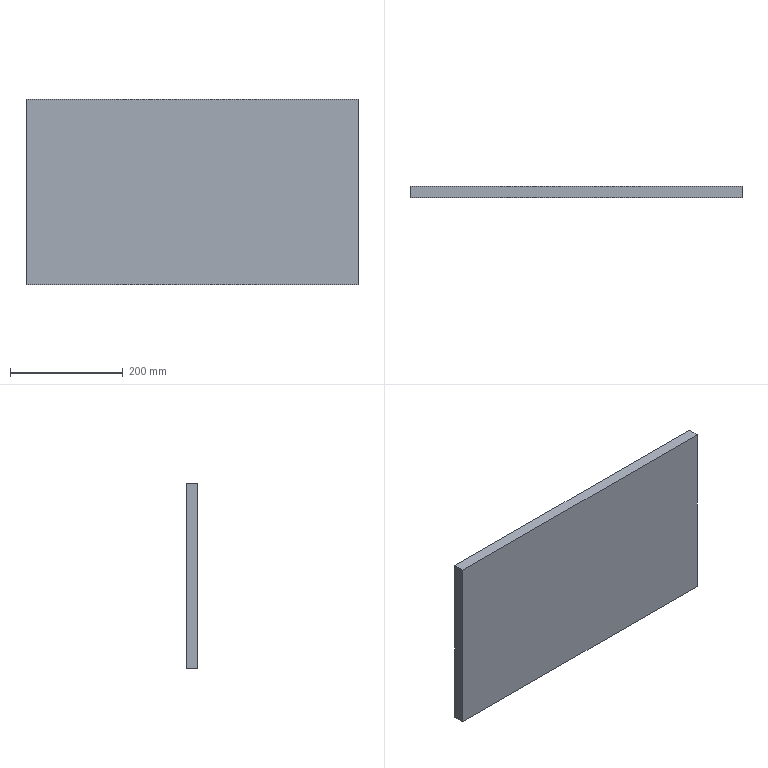Part | STEP file | Light guide plate 001 | 1 solid | 6 faces | box 590 x 20 x 330 mm | volume 3894000 mm3 | plane 6
STEP:
#1=CARTESIAN_POINT('',(0.,0.,0.));
#2=DIRECTION('',(0.,0.,1.));
#3=DIRECTION('',(1.,0.,0.));
#4=AXIS2_PLACEMENT_3D('',#1,#2,#3);
#5=CARTESIAN_POINT('',(295.,0.,165.));
#6=VERTEX_POINT('',#5);
#7=CARTESIAN_POINT('',(295.,0.,-165.));
#8=VERTEX_POINT('',#7);
#9=CARTESIAN_POINT('',(295.,0.,165.));
#10=DIRECTION('',(0.,0.,-1.));
#11=VECTOR('',#10,1.);
#12=LINE('',#9,#11);
#13=CARTESIAN_POINT('',(295.,20.,165.));
#14=DIRECTION('',(-1.,0.,0.));
#15=DIRECTION('',(0.,0.,1.));
#16=AXIS2_PLACEMENT_3D('',#13,#14,#15);
#17=PLANE('',#16);
#18=CARTESIAN_POINT('',(0.,-20.));
#19=DIRECTION('',(-1.,0.));
#20=VECTOR('',#19,1.);
#21=LINE('',#18,#20);
#22=(GEOMETRIC_REPRESENTATION_CONTEXT(2)PARAMETRIC_REPRESENTATION_CONTEXT()REPRESENTATION_CONTEXT('',''));
#23=DEFINITIONAL_REPRESENTATION('',(#21),#22);
#24=PCURVE('',#17,#23);
#25=CARTESIAN_POINT('',(0.,0.,0.));
#26=DIRECTION('',(0.,-1.,0.));
#27=DIRECTION('',(0.,0.,-1.));
#28=AXIS2_PLACEMENT_3D('',#25,#26,#27);
#29=PLANE('',#28);
#30=CARTESIAN_POINT('',(-165.,295.));
#31=DIRECTION('',(1.,0.));
#32=VECTOR('',#31,1.);
#33=LINE('',#30,#32);
#34=(GEOMETRIC_REPRESENTATION_CONTEXT(2)PARAMETRIC_REPRESENTATION_CONTEXT()REPRESENTATION_CONTEXT('',''));
#35=DEFINITIONAL_REPRESENTATION('',(#33),#34);
#36=PCURVE('',#29,#35);
#37=SURFACE_CURVE('',#12,(#24,#36),.PCURVE_S1.);
#38=EDGE_CURVE('',#6,#8,#37,.T.);
#39=ORIENTED_EDGE('',*,*,#38,.T.);
#40=CARTESIAN_POINT('',(295.,20.,-165.));
#41=VERTEX_POINT('',#40);
#42=CARTESIAN_POINT('',(295.,20.,-165.));
#43=DIRECTION('',(0.,-1.,0.));
#44=VECTOR('',#43,1.);
#45=LINE('',#42,#44);
#46=CARTESIAN_POINT('',(-330.,0.));
#47=DIRECTION('',(0.,-1.));
#48=VECTOR('',#47,1.);
#49=LINE('',#46,#48);
#50=(GEOMETRIC_REPRESENTATION_CONTEXT(2)PARAMETRIC_REPRESENTATION_CONTEXT()REPRESENTATION_CONTEXT('',''));
#51=DEFINITIONAL_REPRESENTATION('',(#49),#50);
#52=PCURVE('',#17,#51);
#53=CARTESIAN_POINT('',(-295.,20.,-165.));
#54=DIRECTION('',(0.,0.,1.));
#55=DIRECTION('',(1.,0.,0.));
#56=AXIS2_PLACEMENT_3D('',#53,#54,#55);
#57=PLANE('',#56);
#58=CARTESIAN_POINT('',(590.,0.));
#59=DIRECTION('',(0.,-1.));
#60=VECTOR('',#59,1.);
#61=LINE('',#58,#60);
#62=(GEOMETRIC_REPRESENTATION_CONTEXT(2)PARAMETRIC_REPRESENTATION_CONTEXT()REPRESENTATION_CONTEXT('',''));
#63=DEFINITIONAL_REPRESENTATION('',(#61),#62);
#64=PCURVE('',#57,#63);
#65=SURFACE_CURVE('',#45,(#52,#64),.PCURVE_S1.);
#66=EDGE_CURVE('',#41,#8,#65,.T.);
#67=ORIENTED_EDGE('',*,*,#66,.F.);
#68=CARTESIAN_POINT('',(295.,20.,165.));
#69=VERTEX_POINT('',#68);
#70=CARTESIAN_POINT('',(295.,20.,165.));
#71=DIRECTION('',(0.,0.,-1.));
#72=VECTOR('',#71,1.);
#73=LINE('',#70,#72);
#74=CARTESIAN_POINT('',(0.,0.));
#75=DIRECTION('',(-1.,0.));
#76=VECTOR('',#75,1.);
#77=LINE('',#74,#76);
#78=(GEOMETRIC_REPRESENTATION_CONTEXT(2)PARAMETRIC_REPRESENTATION_CONTEXT()REPRESENTATION_CONTEXT('',''));
#79=DEFINITIONAL_REPRESENTATION('',(#77),#78);
#80=PCURVE('',#17,#79);
#81=CARTESIAN_POINT('',(0.,20.,0.));
#82=DIRECTION('',(0.,-1.,0.));
#83=DIRECTION('',(0.,0.,-1.));
#84=AXIS2_PLACEMENT_3D('',#81,#82,#83);
#85=PLANE('',#84);
#86=CARTESIAN_POINT('',(-165.,295.));
#87=DIRECTION('',(1.,0.));
#88=VECTOR('',#87,1.);
#89=LINE('',#86,#88);
#90=(GEOMETRIC_REPRESENTATION_CONTEXT(2)PARAMETRIC_REPRESENTATION_CONTEXT()REPRESENTATION_CONTEXT('',''));
#91=DEFINITIONAL_REPRESENTATION('',(#89),#90);
#92=PCURVE('',#85,#91);
#93=SURFACE_CURVE('',#73,(#80,#92),.PCURVE_S1.);
#94=EDGE_CURVE('',#69,#41,#93,.T.);
#95=ORIENTED_EDGE('',*,*,#94,.F.);
#96=CARTESIAN_POINT('',(295.,20.,165.));
#97=DIRECTION('',(0.,-1.,0.));
#98=VECTOR('',#97,1.);
#99=LINE('',#96,#98);
#100=CARTESIAN_POINT('',(0.,0.));
#101=DIRECTION('',(0.,-1.));
#102=VECTOR('',#101,1.);
#103=LINE('',#100,#102);
#104=(GEOMETRIC_REPRESENTATION_CONTEXT(2)PARAMETRIC_REPRESENTATION_CONTEXT()REPRESENTATION_CONTEXT('',''));
#105=DEFINITIONAL_REPRESENTATION('',(#103),#104);
#106=PCURVE('',#17,#105);
#107=CARTESIAN_POINT('',(-295.,20.,165.));
#108=DIRECTION('',(0.,0.,-1.));
#109=DIRECTION('',(-1.,0.,0.));
#110=AXIS2_PLACEMENT_3D('',#107,#108,#109);
#111=PLANE('',#110);
#112=CARTESIAN_POINT('',(-590.,0.));
#113=DIRECTION('',(0.,-1.));
#114=VECTOR('',#113,1.);
#115=LINE('',#112,#114);
#116=(GEOMETRIC_REPRESENTATION_CONTEXT(2)PARAMETRIC_REPRESENTATION_CONTEXT()REPRESENTATION_CONTEXT('',''));
#117=DEFINITIONAL_REPRESENTATION('',(#115),#116);
#118=PCURVE('',#111,#117);
#119=SURFACE_CURVE('',#99,(#106,#118),.PCURVE_S1.);
#120=EDGE_CURVE('',#69,#6,#119,.T.);
#121=ORIENTED_EDGE('',*,*,#120,.T.);
#122=EDGE_LOOP('',(#39,#67,#95,#121));
#123=FACE_BOUND('',#122,.T.);
#124=ADVANCED_FACE('',(#123),#17,.F.);
#125=CARTESIAN_POINT('',(-295.,0.,-165.));
#126=VERTEX_POINT('',#125);
#127=CARTESIAN_POINT('',(-295.,0.,-165.));
#128=DIRECTION('',(-1.,0.,0.));
#129=VECTOR('',#128,1.);
#130=LINE('',#127,#129);
#131=CARTESIAN_POINT('',(0.,-20.));
#132=DIRECTION('',(-1.,0.));
#133=VECTOR('',#132,1.);
#134=LINE('',#131,#133);
#135=(GEOMETRIC_REPRESENTATION_CONTEXT(2)PARAMETRIC_REPRESENTATION_CONTEXT()REPRESENTATION_CONTEXT('',''));
#136=DEFINITIONAL_REPRESENTATION('',(#134),#135);
#137=PCURVE('',#57,#136);
#138=CARTESIAN_POINT('',(165.,-295.));
#139=DIRECTION('',(0.,-1.));
#140=VECTOR('',#139,1.);
#141=LINE('',#138,#140);
#142=(GEOMETRIC_REPRESENTATION_CONTEXT(2)PARAMETRIC_REPRESENTATION_CONTEXT()REPRESENTATION_CONTEXT('',''));
#143=DEFINITIONAL_REPRESENTATION('',(#141),#142);
#144=PCURVE('',#29,#143);
#145=SURFACE_CURVE('',#130,(#137,#144),.PCURVE_S1.);
#146=EDGE_CURVE('',#8,#126,#145,.T.);
#147=ORIENTED_EDGE('',*,*,#146,.T.);
#148=CARTESIAN_POINT('',(-295.,20.,-165.));
#149=VERTEX_POINT('',#148);
#150=CARTESIAN_POINT('',(-295.,20.,-165.));
#151=DIRECTION('',(0.,-1.,0.));
#152=VECTOR('',#151,1.);
#153=LINE('',#150,#152);
#154=CARTESIAN_POINT('',(0.,0.));
#155=DIRECTION('',(0.,-1.));
#156=VECTOR('',#155,1.);
#157=LINE('',#154,#156);
#158=(GEOMETRIC_REPRESENTATION_CONTEXT(2)PARAMETRIC_REPRESENTATION_CONTEXT()REPRESENTATION_CONTEXT('',''));
#159=DEFINITIONAL_REPRESENTATION('',(#157),#158);
#160=PCURVE('',#57,#159);
#161=CARTESIAN_POINT('',(-295.,20.,165.));
#162=DIRECTION('',(1.,0.,0.));
#163=DIRECTION('',(0.,0.,-1.));
#164=AXIS2_PLACEMENT_3D('',#161,#162,#163);
#165=PLANE('',#164);
#166=CARTESIAN_POINT('',(330.,0.));
#167=DIRECTION('',(0.,-1.));
#168=VECTOR('',#167,1.);
#169=LINE('',#166,#168);
#170=(GEOMETRIC_REPRESENTATION_CONTEXT(2)PARAMETRIC_REPRESENTATION_CONTEXT()REPRESENTATION_CONTEXT('',''));
#171=DEFINITIONAL_REPRESENTATION('',(#169),#170);
#172=PCURVE('',#165,#171);
#173=SURFACE_CURVE('',#153,(#160,#172),.PCURVE_S1.);
#174=EDGE_CURVE('',#149,#126,#173,.T.);
#175=ORIENTED_EDGE('',*,*,#174,.F.);
#176=CARTESIAN_POINT('',(-295.,20.,-165.));
#177=DIRECTION('',(-1.,0.,0.));
#178=VECTOR('',#177,1.);
#179=LINE('',#176,#178);
#180=CARTESIAN_POINT('',(0.,0.));
#181=DIRECTION('',(-1.,0.));
#182=VECTOR('',#181,1.);
#183=LINE('',#180,#182);
#184=(GEOMETRIC_REPRESENTATION_CONTEXT(2)PARAMETRIC_REPRESENTATION_CONTEXT()REPRESENTATION_CONTEXT('',''));
#185=DEFINITIONAL_REPRESENTATION('',(#183),#184);
#186=PCURVE('',#57,#185);
#187=CARTESIAN_POINT('',(165.,-295.));
#188=DIRECTION('',(0.,-1.));
#189=VECTOR('',#188,1.);
#190=LINE('',#187,#189);
#191=(GEOMETRIC_REPRESENTATION_CONTEXT(2)PARAMETRIC_REPRESENTATION_CONTEXT()REPRESENTATION_CONTEXT('',''));
#192=DEFINITIONAL_REPRESENTATION('',(#190),#191);
#193=PCURVE('',#85,#192);
#194=SURFACE_CURVE('',#179,(#186,#193),.PCURVE_S1.);
#195=EDGE_CURVE('',#41,#149,#194,.T.);
#196=ORIENTED_EDGE('',*,*,#195,.F.);
#197=ORIENTED_EDGE('',*,*,#66,.T.);
#198=EDGE_LOOP('',(#147,#175,#196,#197));
#199=FACE_BOUND('',#198,.T.);
#200=ADVANCED_FACE('',(#199),#57,.F.);
#201=CARTESIAN_POINT('',(-295.,0.,165.));
#202=VERTEX_POINT('',#201);
#203=CARTESIAN_POINT('',(-295.,0.,165.));
#204=DIRECTION('',(0.,0.,1.));
#205=VECTOR('',#204,1.);
#206=LINE('',#203,#205);
#207=CARTESIAN_POINT('',(0.,-20.));
#208=DIRECTION('',(-1.,0.));
#209=VECTOR('',#208,1.);
#210=LINE('',#207,#209);
#211=(GEOMETRIC_REPRESENTATION_CONTEXT(2)PARAMETRIC_REPRESENTATION_CONTEXT()REPRESENTATION_CONTEXT('',''));
#212=DEFINITIONAL_REPRESENTATION('',(#210),#211);
#213=PCURVE('',#165,#212);
#214=CARTESIAN_POINT('',(-165.,-295.));
#215=DIRECTION('',(-1.,0.));
#216=VECTOR('',#215,1.);
#217=LINE('',#214,#216);
#218=(GEOMETRIC_REPRESENTATION_CONTEXT(2)PARAMETRIC_REPRESENTATION_CONTEXT()REPRESENTATION_CONTEXT('',''));
#219=DEFINITIONAL_REPRESENTATION('',(#217),#218);
#220=PCURVE('',#29,#219);
#221=SURFACE_CURVE('',#206,(#213,#220),.PCURVE_S1.);
#222=EDGE_CURVE('',#126,#202,#221,.T.);
#223=ORIENTED_EDGE('',*,*,#222,.T.);
#224=CARTESIAN_POINT('',(-295.,20.,165.));
#225=VERTEX_POINT('',#224);
#226=CARTESIAN_POINT('',(-295.,20.,165.));
#227=DIRECTION('',(0.,-1.,0.));
#228=VECTOR('',#227,1.);
#229=LINE('',#226,#228);
#230=CARTESIAN_POINT('',(0.,0.));
#231=DIRECTION('',(0.,-1.));
#232=VECTOR('',#231,1.);
#233=LINE('',#230,#232);
#234=(GEOMETRIC_REPRESENTATION_CONTEXT(2)PARAMETRIC_REPRESENTATION_CONTEXT()REPRESENTATION_CONTEXT('',''));
#235=DEFINITIONAL_REPRESENTATION('',(#233),#234);
#236=PCURVE('',#165,#235);
#237=CARTESIAN_POINT('',(0.,0.));
#238=DIRECTION('',(0.,-1.));
#239=VECTOR('',#238,1.);
#240=LINE('',#237,#239);
#241=(GEOMETRIC_REPRESENTATION_CONTEXT(2)PARAMETRIC_REPRESENTATION_CONTEXT()REPRESENTATION_CONTEXT('',''));
#242=DEFINITIONAL_REPRESENTATION('',(#240),#241);
#243=PCURVE('',#111,#242);
#244=SURFACE_CURVE('',#229,(#236,#243),.PCURVE_S1.);
#245=EDGE_CURVE('',#225,#202,#244,.T.);
#246=ORIENTED_EDGE('',*,*,#245,.F.);
#247=CARTESIAN_POINT('',(-295.,20.,165.));
#248=DIRECTION('',(0.,0.,1.));
#249=VECTOR('',#248,1.);
#250=LINE('',#247,#249);
#251=CARTESIAN_POINT('',(0.,0.));
#252=DIRECTION('',(-1.,0.));
#253=VECTOR('',#252,1.);
#254=LINE('',#251,#253);
#255=(GEOMETRIC_REPRESENTATION_CONTEXT(2)PARAMETRIC_REPRESENTATION_CONTEXT()REPRESENTATION_CONTEXT('',''));
#256=DEFINITIONAL_REPRESENTATION('',(#254),#255);
#257=PCURVE('',#165,#256);
#258=CARTESIAN_POINT('',(-165.,-295.));
#259=DIRECTION('',(-1.,0.));
#260=VECTOR('',#259,1.);
#261=LINE('',#258,#260);
#262=(GEOMETRIC_REPRESENTATION_CONTEXT(2)PARAMETRIC_REPRESENTATION_CONTEXT()REPRESENTATION_CONTEXT('',''));
#263=DEFINITIONAL_REPRESENTATION('',(#261),#262);
#264=PCURVE('',#85,#263);
#265=SURFACE_CURVE('',#250,(#257,#264),.PCURVE_S1.);
#266=EDGE_CURVE('',#149,#225,#265,.T.);
#267=ORIENTED_EDGE('',*,*,#266,.F.);
#268=ORIENTED_EDGE('',*,*,#174,.T.);
#269=EDGE_LOOP('',(#223,#246,#267,#268));
#270=FACE_BOUND('',#269,.T.);
#271=ADVANCED_FACE('',(#270),#165,.F.);
#272=CARTESIAN_POINT('',(-295.,0.,165.));
#273=DIRECTION('',(1.,0.,0.));
#274=VECTOR('',#273,1.);
#275=LINE('',#272,#274);
#276=CARTESIAN_POINT('',(0.,-20.));
#277=DIRECTION('',(-1.,0.));
#278=VECTOR('',#277,1.);
#279=LINE('',#276,#278);
#280=(GEOMETRIC_REPRESENTATION_CONTEXT(2)PARAMETRIC_REPRESENTATION_CONTEXT()REPRESENTATION_CONTEXT('',''));
#281=DEFINITIONAL_REPRESENTATION('',(#279),#280);
#282=PCURVE('',#111,#281);
#283=CARTESIAN_POINT('',(-165.,-295.));
#284=DIRECTION('',(0.,1.));
#285=VECTOR('',#284,1.);
#286=LINE('',#283,#285);
#287=(GEOMETRIC_REPRESENTATION_CONTEXT(2)PARAMETRIC_REPRESENTATION_CONTEXT()REPRESENTATION_CONTEXT('',''));
#288=DEFINITIONAL_REPRESENTATION('',(#286),#287);
#289=PCURVE('',#29,#288);
#290=SURFACE_CURVE('',#275,(#282,#289),.PCURVE_S1.);
#291=EDGE_CURVE('',#202,#6,#290,.T.);
#292=ORIENTED_EDGE('',*,*,#291,.T.);
#293=ORIENTED_EDGE('',*,*,#120,.F.);
#294=CARTESIAN_POINT('',(-295.,20.,165.));
#295=DIRECTION('',(1.,0.,0.));
#296=VECTOR('',#295,1.);
#297=LINE('',#294,#296);
#298=CARTESIAN_POINT('',(0.,0.));
#299=DIRECTION('',(-1.,0.));
#300=VECTOR('',#299,1.);
#301=LINE('',#298,#300);
#302=(GEOMETRIC_REPRESENTATION_CONTEXT(2)PARAMETRIC_REPRESENTATION_CONTEXT()REPRESENTATION_CONTEXT('',''));
#303=DEFINITIONAL_REPRESENTATION('',(#301),#302);
#304=PCURVE('',#111,#303);
#305=CARTESIAN_POINT('',(-165.,-295.));
#306=DIRECTION('',(0.,1.));
#307=VECTOR('',#306,1.);
#308=LINE('',#305,#307);
#309=(GEOMETRIC_REPRESENTATION_CONTEXT(2)PARAMETRIC_REPRESENTATION_CONTEXT()REPRESENTATION_CONTEXT('',''));
#310=DEFINITIONAL_REPRESENTATION('',(#308),#309);
#311=PCURVE('',#85,#310);
#312=SURFACE_CURVE('',#297,(#304,#311),.PCURVE_S1.);
#313=EDGE_CURVE('',#225,#69,#312,.T.);
#314=ORIENTED_EDGE('',*,*,#313,.F.);
#315=ORIENTED_EDGE('',*,*,#245,.T.);
#316=EDGE_LOOP('',(#292,#293,#314,#315));
#317=FACE_BOUND('',#316,.T.);
#318=ADVANCED_FACE('',(#317),#111,.F.);
#319=ORIENTED_EDGE('',*,*,#94,.T.);
#320=ORIENTED_EDGE('',*,*,#195,.T.);
#321=ORIENTED_EDGE('',*,*,#266,.T.);
#322=ORIENTED_EDGE('',*,*,#313,.T.);
#323=EDGE_LOOP('',(#319,#320,#321,#322));
#324=FACE_BOUND('',#323,.T.);
#325=ADVANCED_FACE('',(#324),#85,.F.);
#326=ORIENTED_EDGE('',*,*,#38,.F.);
#327=ORIENTED_EDGE('',*,*,#291,.F.);
#328=ORIENTED_EDGE('',*,*,#222,.F.);
#329=ORIENTED_EDGE('',*,*,#146,.F.);
#330=EDGE_LOOP('',(#326,#327,#328,#329));
#331=FACE_BOUND('',#330,.T.);
#332=ADVANCED_FACE('',(#331),#29,.T.);
#333=CLOSED_SHELL('',(#124,#200,#271,#318,#325,#332));
#334=MANIFOLD_SOLID_BREP('',#333);
#335=(LENGTH_UNIT()NAMED_UNIT(*)SI_UNIT(.MILLI.,.METRE.));
#336=UNCERTAINTY_MEASURE_WITH_UNIT(LENGTH_MEASURE(0.0000001),#335,'','');
#337=(NAMED_UNIT(*)PLANE_ANGLE_UNIT()SI_UNIT($,.RADIAN.));
#338=(NAMED_UNIT(*)SI_UNIT($,.STERADIAN.)SOLID_ANGLE_UNIT());
#339=(GEOMETRIC_REPRESENTATION_CONTEXT(3)GLOBAL_UNCERTAINTY_ASSIGNED_CONTEXT((#336))GLOBAL_UNIT_ASSIGNED_CONTEXT((#335,#337,#338))REPRESENTATION_CONTEXT('',''));
#340=ADVANCED_BREP_SHAPE_REPRESENTATION('',(#4,#334),#339);